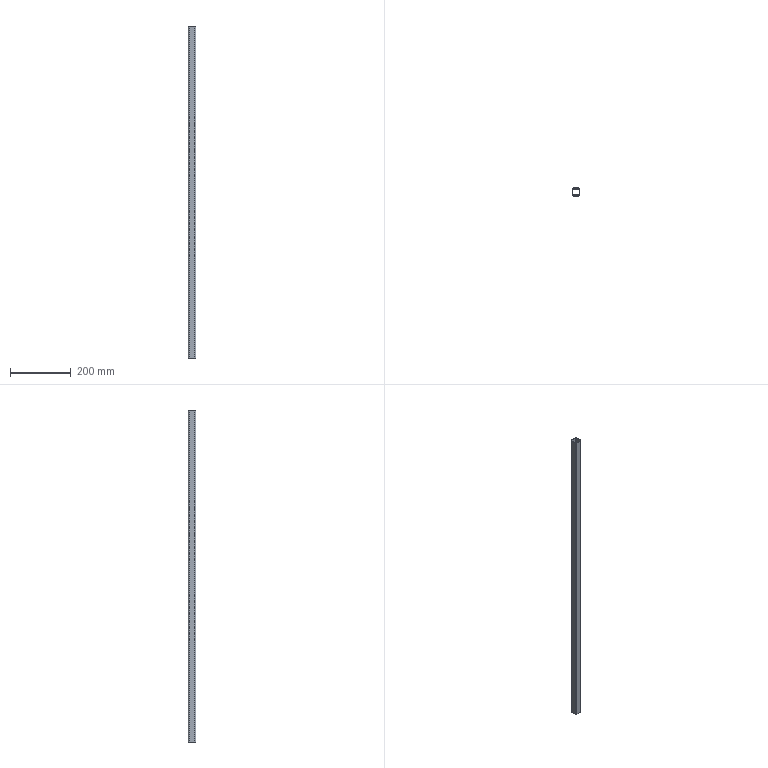Part | SolidWorks | features Extrusion 1 | 1 solid | 18 faces | box 25 x 25 x 1094 mm | volume 190027 mm3 | plane 10 | cylinder 8 | commonest cylinder face diameters 4 x4 8 x4
STEP:
#1=CARTESIAN_POINT('',(12.5,8.5,1094.));
#2=VERTEX_POINT('',#1);
#3=CARTESIAN_POINT('',(8.5,12.5,1094.));
#4=VERTEX_POINT('',#3);
#5=CARTESIAN_POINT('',(8.5,8.5,1094.));
#6=DIRECTION('',(0.,0.,1.));
#7=DIRECTION('',(1.,0.,0.));
#8=AXIS2_PLACEMENT_3D('',#5,#6,#7);
#9=CIRCLE('',#8,4.);
#10=EDGE_CURVE('',#2,#4,#9,.T.);
#11=ORIENTED_EDGE('',*,*,#10,.T.);
#12=CARTESIAN_POINT('',(-8.5,12.5,1094.));
#13=VERTEX_POINT('',#12);
#14=CARTESIAN_POINT('',(8.5,12.5,1094.));
#15=DIRECTION('',(-1.,0.,0.));
#16=VECTOR('',#15,1000.);
#17=LINE('',#14,#16);
#18=EDGE_CURVE('',#4,#13,#17,.T.);
#19=ORIENTED_EDGE('',*,*,#18,.T.);
#20=CARTESIAN_POINT('',(-12.5,8.5,1094.));
#21=VERTEX_POINT('',#20);
#22=CARTESIAN_POINT('',(-8.5,8.5,1094.));
#23=DIRECTION('',(0.,0.,1.));
#24=DIRECTION('',(1.,0.,0.));
#25=AXIS2_PLACEMENT_3D('',#22,#23,#24);
#26=CIRCLE('',#25,4.);
#27=EDGE_CURVE('',#13,#21,#26,.T.);
#28=ORIENTED_EDGE('',*,*,#27,.T.);
#29=CARTESIAN_POINT('',(-12.5,-8.5,1094.));
#30=VERTEX_POINT('',#29);
#31=CARTESIAN_POINT('',(-12.5,-8.5,1094.));
#32=DIRECTION('',(0.,-1.,0.));
#33=VECTOR('',#32,1000.);
#34=LINE('',#31,#33);
#35=EDGE_CURVE('',#21,#30,#34,.T.);
#36=ORIENTED_EDGE('',*,*,#35,.T.);
#37=CARTESIAN_POINT('',(-8.5,-12.5,1094.));
#38=VERTEX_POINT('',#37);
#39=CARTESIAN_POINT('',(-8.5,-8.5,1094.));
#40=DIRECTION('',(0.,0.,1.));
#41=DIRECTION('',(1.,0.,0.));
#42=AXIS2_PLACEMENT_3D('',#39,#40,#41);
#43=CIRCLE('',#42,4.);
#44=EDGE_CURVE('',#30,#38,#43,.T.);
#45=ORIENTED_EDGE('',*,*,#44,.T.);
#46=CARTESIAN_POINT('',(8.5,-12.5,1094.));
#47=VERTEX_POINT('',#46);
#48=CARTESIAN_POINT('',(-8.5,-12.5,1094.));
#49=DIRECTION('',(1.,0.,0.));
#50=VECTOR('',#49,1000.);
#51=LINE('',#48,#50);
#52=EDGE_CURVE('',#38,#47,#51,.T.);
#53=ORIENTED_EDGE('',*,*,#52,.T.);
#54=CARTESIAN_POINT('',(12.5,-8.5,1094.));
#55=VERTEX_POINT('',#54);
#56=CARTESIAN_POINT('',(8.5,-8.5,1094.));
#57=DIRECTION('',(0.,0.,1.));
#58=DIRECTION('',(1.,0.,0.));
#59=AXIS2_PLACEMENT_3D('',#56,#57,#58);
#60=CIRCLE('',#59,4.);
#61=EDGE_CURVE('',#47,#55,#60,.T.);
#62=ORIENTED_EDGE('',*,*,#61,.T.);
#63=CARTESIAN_POINT('',(12.5,8.5,1094.));
#64=DIRECTION('',(0.,1.,0.));
#65=VECTOR('',#64,1000.);
#66=LINE('',#63,#65);
#67=EDGE_CURVE('',#55,#2,#66,.T.);
#68=ORIENTED_EDGE('',*,*,#67,.T.);
#69=EDGE_LOOP('',(#11,#19,#28,#36,#45,#53,#62,#68));
#70=FACE_OUTER_BOUND('',#69,.T.);
#71=CARTESIAN_POINT('',(-10.5,8.5,1094.));
#72=VERTEX_POINT('',#71);
#73=CARTESIAN_POINT('',(-10.5,-8.5,1094.));
#74=VERTEX_POINT('',#73);
#75=CARTESIAN_POINT('',(-10.5,-8.5,1094.));
#76=DIRECTION('',(0.,-1.,0.));
#77=VECTOR('',#76,1000.);
#78=LINE('',#75,#77);
#79=EDGE_CURVE('',#72,#74,#78,.T.);
#80=ORIENTED_EDGE('',*,*,#79,.F.);
#81=CARTESIAN_POINT('',(-8.5,10.5,1094.));
#82=VERTEX_POINT('',#81);
#83=CARTESIAN_POINT('',(-8.5,8.5,1094.));
#84=DIRECTION('',(0.,0.,1.));
#85=DIRECTION('',(1.,0.,0.));
#86=AXIS2_PLACEMENT_3D('',#83,#84,#85);
#87=CIRCLE('',#86,2.);
#88=EDGE_CURVE('',#82,#72,#87,.T.);
#89=ORIENTED_EDGE('',*,*,#88,.F.);
#90=CARTESIAN_POINT('',(8.5,10.5,1094.));
#91=VERTEX_POINT('',#90);
#92=CARTESIAN_POINT('',(8.5,10.5,1094.));
#93=DIRECTION('',(-1.,0.,0.));
#94=VECTOR('',#93,1000.);
#95=LINE('',#92,#94);
#96=EDGE_CURVE('',#91,#82,#95,.T.);
#97=ORIENTED_EDGE('',*,*,#96,.F.);
#98=CARTESIAN_POINT('',(10.5,8.5,1094.));
#99=VERTEX_POINT('',#98);
#100=CARTESIAN_POINT('',(8.5,8.5,1094.));
#101=DIRECTION('',(0.,0.,1.));
#102=DIRECTION('',(1.,0.,0.));
#103=AXIS2_PLACEMENT_3D('',#100,#101,#102);
#104=CIRCLE('',#103,2.);
#105=EDGE_CURVE('',#99,#91,#104,.T.);
#106=ORIENTED_EDGE('',*,*,#105,.F.);
#107=CARTESIAN_POINT('',(10.5,-8.5,1094.));
#108=VERTEX_POINT('',#107);
#109=CARTESIAN_POINT('',(10.5,8.5,1094.));
#110=DIRECTION('',(0.,1.,0.));
#111=VECTOR('',#110,1000.);
#112=LINE('',#109,#111);
#113=EDGE_CURVE('',#108,#99,#112,.T.);
#114=ORIENTED_EDGE('',*,*,#113,.F.);
#115=CARTESIAN_POINT('',(8.5,-10.5,1094.));
#116=VERTEX_POINT('',#115);
#117=CARTESIAN_POINT('',(8.5,-8.5,1094.));
#118=DIRECTION('',(0.,0.,1.));
#119=DIRECTION('',(1.,0.,0.));
#120=AXIS2_PLACEMENT_3D('',#117,#118,#119);
#121=CIRCLE('',#120,2.);
#122=EDGE_CURVE('',#116,#108,#121,.T.);
#123=ORIENTED_EDGE('',*,*,#122,.F.);
#124=CARTESIAN_POINT('',(-8.5,-10.5,1094.));
#125=VERTEX_POINT('',#124);
#126=CARTESIAN_POINT('',(-8.5,-10.5,1094.));
#127=DIRECTION('',(1.,0.,0.));
#128=VECTOR('',#127,1000.);
#129=LINE('',#126,#128);
#130=EDGE_CURVE('',#125,#116,#129,.T.);
#131=ORIENTED_EDGE('',*,*,#130,.F.);
#132=CARTESIAN_POINT('',(-8.5,-8.5,1094.));
#133=DIRECTION('',(0.,0.,1.));
#134=DIRECTION('',(1.,0.,0.));
#135=AXIS2_PLACEMENT_3D('',#132,#133,#134);
#136=CIRCLE('',#135,2.);
#137=EDGE_CURVE('',#74,#125,#136,.T.);
#138=ORIENTED_EDGE('',*,*,#137,.F.);
#139=EDGE_LOOP('',(#80,#89,#97,#106,#114,#123,#131,#138));
#140=FACE_BOUND('',#139,.T.);
#141=CARTESIAN_POINT('',(8.5,8.5,1094.));
#142=DIRECTION('',(0.,0.,1.));
#143=DIRECTION('',(1.,0.,0.));
#144=AXIS2_PLACEMENT_3D('',#141,#142,#143);
#145=PLANE('',#144);
#146=ADVANCED_FACE('',(#70,#140),#145,.T.);
#147=CARTESIAN_POINT('',(12.5,8.5,0.));
#148=VERTEX_POINT('',#147);
#149=CARTESIAN_POINT('',(8.5,12.5,0.));
#150=VERTEX_POINT('',#149);
#151=CARTESIAN_POINT('',(8.5,8.5,0.));
#152=DIRECTION('',(0.,0.,1.));
#153=DIRECTION('',(1.,0.,0.));
#154=AXIS2_PLACEMENT_3D('',#151,#152,#153);
#155=CIRCLE('',#154,4.);
#156=EDGE_CURVE('',#148,#150,#155,.T.);
#157=ORIENTED_EDGE('',*,*,#156,.F.);
#158=CARTESIAN_POINT('',(12.5,-8.5,0.));
#159=VERTEX_POINT('',#158);
#160=CARTESIAN_POINT('',(12.5,8.5,0.));
#161=DIRECTION('',(0.,1.,0.));
#162=VECTOR('',#161,1000.);
#163=LINE('',#160,#162);
#164=EDGE_CURVE('',#159,#148,#163,.T.);
#165=ORIENTED_EDGE('',*,*,#164,.F.);
#166=CARTESIAN_POINT('',(8.5,-12.5,0.));
#167=VERTEX_POINT('',#166);
#168=CARTESIAN_POINT('',(8.5,-8.5,0.));
#169=DIRECTION('',(0.,0.,1.));
#170=DIRECTION('',(1.,0.,0.));
#171=AXIS2_PLACEMENT_3D('',#168,#169,#170);
#172=CIRCLE('',#171,4.);
#173=EDGE_CURVE('',#167,#159,#172,.T.);
#174=ORIENTED_EDGE('',*,*,#173,.F.);
#175=CARTESIAN_POINT('',(-8.5,-12.5,0.));
#176=VERTEX_POINT('',#175);
#177=CARTESIAN_POINT('',(-8.5,-12.5,0.));
#178=DIRECTION('',(1.,0.,0.));
#179=VECTOR('',#178,1000.);
#180=LINE('',#177,#179);
#181=EDGE_CURVE('',#176,#167,#180,.T.);
#182=ORIENTED_EDGE('',*,*,#181,.F.);
#183=CARTESIAN_POINT('',(-12.5,-8.5,0.));
#184=VERTEX_POINT('',#183);
#185=CARTESIAN_POINT('',(-8.5,-8.5,0.));
#186=DIRECTION('',(0.,0.,1.));
#187=DIRECTION('',(1.,0.,0.));
#188=AXIS2_PLACEMENT_3D('',#185,#186,#187);
#189=CIRCLE('',#188,4.);
#190=EDGE_CURVE('',#184,#176,#189,.T.);
#191=ORIENTED_EDGE('',*,*,#190,.F.);
#192=CARTESIAN_POINT('',(-12.5,8.5,0.));
#193=VERTEX_POINT('',#192);
#194=CARTESIAN_POINT('',(-12.5,-8.5,0.));
#195=DIRECTION('',(0.,-1.,0.));
#196=VECTOR('',#195,1000.);
#197=LINE('',#194,#196);
#198=EDGE_CURVE('',#193,#184,#197,.T.);
#199=ORIENTED_EDGE('',*,*,#198,.F.);
#200=CARTESIAN_POINT('',(-8.5,12.5,0.));
#201=VERTEX_POINT('',#200);
#202=CARTESIAN_POINT('',(-8.5,8.5,0.));
#203=DIRECTION('',(0.,0.,1.));
#204=DIRECTION('',(1.,0.,0.));
#205=AXIS2_PLACEMENT_3D('',#202,#203,#204);
#206=CIRCLE('',#205,4.);
#207=EDGE_CURVE('',#201,#193,#206,.T.);
#208=ORIENTED_EDGE('',*,*,#207,.F.);
#209=CARTESIAN_POINT('',(8.5,12.5,0.));
#210=DIRECTION('',(-1.,0.,0.));
#211=VECTOR('',#210,1000.);
#212=LINE('',#209,#211);
#213=EDGE_CURVE('',#150,#201,#212,.T.);
#214=ORIENTED_EDGE('',*,*,#213,.F.);
#215=EDGE_LOOP('',(#157,#165,#174,#182,#191,#199,#208,#214));
#216=FACE_OUTER_BOUND('',#215,.T.);
#217=CARTESIAN_POINT('',(-8.5,10.5,0.));
#218=VERTEX_POINT('',#217);
#219=CARTESIAN_POINT('',(-10.5,8.5,0.));
#220=VERTEX_POINT('',#219);
#221=CARTESIAN_POINT('',(-8.5,8.5,0.));
#222=DIRECTION('',(0.,0.,1.));
#223=DIRECTION('',(1.,0.,0.));
#224=AXIS2_PLACEMENT_3D('',#221,#222,#223);
#225=CIRCLE('',#224,2.);
#226=EDGE_CURVE('',#218,#220,#225,.T.);
#227=ORIENTED_EDGE('',*,*,#226,.T.);
#228=CARTESIAN_POINT('',(-10.5,-8.5,0.));
#229=VERTEX_POINT('',#228);
#230=CARTESIAN_POINT('',(-10.5,-8.5,0.));
#231=DIRECTION('',(0.,-1.,0.));
#232=VECTOR('',#231,1000.);
#233=LINE('',#230,#232);
#234=EDGE_CURVE('',#220,#229,#233,.T.);
#235=ORIENTED_EDGE('',*,*,#234,.T.);
#236=CARTESIAN_POINT('',(-8.5,-10.5,0.));
#237=VERTEX_POINT('',#236);
#238=CARTESIAN_POINT('',(-8.5,-8.5,0.));
#239=DIRECTION('',(0.,0.,1.));
#240=DIRECTION('',(1.,0.,0.));
#241=AXIS2_PLACEMENT_3D('',#238,#239,#240);
#242=CIRCLE('',#241,2.);
#243=EDGE_CURVE('',#229,#237,#242,.T.);
#244=ORIENTED_EDGE('',*,*,#243,.T.);
#245=CARTESIAN_POINT('',(8.5,-10.5,0.));
#246=VERTEX_POINT('',#245);
#247=CARTESIAN_POINT('',(-8.5,-10.5,0.));
#248=DIRECTION('',(1.,0.,0.));
#249=VECTOR('',#248,1000.);
#250=LINE('',#247,#249);
#251=EDGE_CURVE('',#237,#246,#250,.T.);
#252=ORIENTED_EDGE('',*,*,#251,.T.);
#253=CARTESIAN_POINT('',(10.5,-8.5,0.));
#254=VERTEX_POINT('',#253);
#255=CARTESIAN_POINT('',(8.5,-8.5,0.));
#256=DIRECTION('',(0.,0.,1.));
#257=DIRECTION('',(1.,0.,0.));
#258=AXIS2_PLACEMENT_3D('',#255,#256,#257);
#259=CIRCLE('',#258,2.);
#260=EDGE_CURVE('',#246,#254,#259,.T.);
#261=ORIENTED_EDGE('',*,*,#260,.T.);
#262=CARTESIAN_POINT('',(10.5,8.5,0.));
#263=VERTEX_POINT('',#262);
#264=CARTESIAN_POINT('',(10.5,8.5,0.));
#265=DIRECTION('',(0.,1.,0.));
#266=VECTOR('',#265,1000.);
#267=LINE('',#264,#266);
#268=EDGE_CURVE('',#254,#263,#267,.T.);
#269=ORIENTED_EDGE('',*,*,#268,.T.);
#270=CARTESIAN_POINT('',(8.5,10.5,0.));
#271=VERTEX_POINT('',#270);
#272=CARTESIAN_POINT('',(8.5,8.5,0.));
#273=DIRECTION('',(0.,0.,1.));
#274=DIRECTION('',(1.,0.,0.));
#275=AXIS2_PLACEMENT_3D('',#272,#273,#274);
#276=CIRCLE('',#275,2.);
#277=EDGE_CURVE('',#263,#271,#276,.T.);
#278=ORIENTED_EDGE('',*,*,#277,.T.);
#279=CARTESIAN_POINT('',(8.5,10.5,0.));
#280=DIRECTION('',(-1.,0.,0.));
#281=VECTOR('',#280,1000.);
#282=LINE('',#279,#281);
#283=EDGE_CURVE('',#271,#218,#282,.T.);
#284=ORIENTED_EDGE('',*,*,#283,.T.);
#285=EDGE_LOOP('',(#227,#235,#244,#252,#261,#269,#278,#284));
#286=FACE_BOUND('',#285,.T.);
#287=CARTESIAN_POINT('',(8.5,8.5,0.));
#288=DIRECTION('',(0.,0.,1.));
#289=DIRECTION('',(1.,0.,0.));
#290=AXIS2_PLACEMENT_3D('',#287,#288,#289);
#291=PLANE('',#290);
#292=ADVANCED_FACE('',(#216,#286),#291,.F.);
#293=ORIENTED_EDGE('',*,*,#156,.T.);
#294=CARTESIAN_POINT('',(8.5,12.5,1094.));
#295=DIRECTION('',(0.,0.,-1.));
#296=VECTOR('',#295,1000.);
#297=LINE('',#294,#296);
#298=EDGE_CURVE('',#4,#150,#297,.T.);
#299=ORIENTED_EDGE('',*,*,#298,.F.);
#300=ORIENTED_EDGE('',*,*,#10,.F.);
#301=CARTESIAN_POINT('',(12.5,8.5,1094.));
#302=DIRECTION('',(0.,0.,-1.));
#303=VECTOR('',#302,1000.);
#304=LINE('',#301,#303);
#305=EDGE_CURVE('',#2,#148,#304,.T.);
#306=ORIENTED_EDGE('',*,*,#305,.T.);
#307=EDGE_LOOP('',(#293,#299,#300,#306));
#308=FACE_OUTER_BOUND('',#307,.T.);
#309=CARTESIAN_POINT('',(8.5,8.5,1094.));
#310=DIRECTION('',(0.,0.,-1.));
#311=DIRECTION('',(-1.,0.,0.));
#312=AXIS2_PLACEMENT_3D('',#309,#310,#311);
#313=CYLINDRICAL_SURFACE('',#312,4.);
#314=ADVANCED_FACE('',(#308),#313,.T.);
#315=ORIENTED_EDGE('',*,*,#213,.T.);
#316=CARTESIAN_POINT('',(-8.5,12.5,1094.));
#317=DIRECTION('',(0.,0.,-1.));
#318=VECTOR('',#317,1000.);
#319=LINE('',#316,#318);
#320=EDGE_CURVE('',#13,#201,#319,.T.);
#321=ORIENTED_EDGE('',*,*,#320,.F.);
#322=ORIENTED_EDGE('',*,*,#18,.F.);
#323=ORIENTED_EDGE('',*,*,#298,.T.);
#324=EDGE_LOOP('',(#315,#321,#322,#323));
#325=FACE_OUTER_BOUND('',#324,.T.);
#326=CARTESIAN_POINT('',(8.5,12.5,1094.));
#327=DIRECTION('',(0.,-1.,0.));
#328=DIRECTION('',(0.,0.,-1.));
#329=AXIS2_PLACEMENT_3D('',#326,#327,#328);
#330=PLANE('',#329);
#331=ADVANCED_FACE('',(#325),#330,.F.);
#332=ORIENTED_EDGE('',*,*,#207,.T.);
#333=CARTESIAN_POINT('',(-12.5,8.5,1094.));
#334=DIRECTION('',(0.,0.,-1.));
#335=VECTOR('',#334,1000.);
#336=LINE('',#333,#335);
#337=EDGE_CURVE('',#21,#193,#336,.T.);
#338=ORIENTED_EDGE('',*,*,#337,.F.);
#339=ORIENTED_EDGE('',*,*,#27,.F.);
#340=ORIENTED_EDGE('',*,*,#320,.T.);
#341=EDGE_LOOP('',(#332,#338,#339,#340));
#342=FACE_OUTER_BOUND('',#341,.T.);
#343=CARTESIAN_POINT('',(-8.5,8.5,1094.));
#344=DIRECTION('',(0.,0.,-1.));
#345=DIRECTION('',(-1.,0.,0.));
#346=AXIS2_PLACEMENT_3D('',#343,#344,#345);
#347=CYLINDRICAL_SURFACE('',#346,4.);
#348=ADVANCED_FACE('',(#342),#347,.T.);
#349=ORIENTED_EDGE('',*,*,#198,.T.);
#350=CARTESIAN_POINT('',(-12.5,-8.5,1094.));
#351=DIRECTION('',(0.,0.,-1.));
#352=VECTOR('',#351,1000.);
#353=LINE('',#350,#352);
#354=EDGE_CURVE('',#30,#184,#353,.T.);
#355=ORIENTED_EDGE('',*,*,#354,.F.);
#356=ORIENTED_EDGE('',*,*,#35,.F.);
#357=ORIENTED_EDGE('',*,*,#337,.T.);
#358=EDGE_LOOP('',(#349,#355,#356,#357));
#359=FACE_OUTER_BOUND('',#358,.T.);
#360=CARTESIAN_POINT('',(-12.5,-8.5,1094.));
#361=DIRECTION('',(1.,0.,0.));
#362=DIRECTION('',(0.,0.,-1.));
#363=AXIS2_PLACEMENT_3D('',#360,#361,#362);
#364=PLANE('',#363);
#365=ADVANCED_FACE('',(#359),#364,.F.);
#366=ORIENTED_EDGE('',*,*,#190,.T.);
#367=CARTESIAN_POINT('',(-8.5,-12.5,1094.));
#368=DIRECTION('',(0.,0.,-1.));
#369=VECTOR('',#368,1000.);
#370=LINE('',#367,#369);
#371=EDGE_CURVE('',#38,#176,#370,.T.);
#372=ORIENTED_EDGE('',*,*,#371,.F.);
#373=ORIENTED_EDGE('',*,*,#44,.F.);
#374=ORIENTED_EDGE('',*,*,#354,.T.);
#375=EDGE_LOOP('',(#366,#372,#373,#374));
#376=FACE_OUTER_BOUND('',#375,.T.);
#377=CARTESIAN_POINT('',(-8.5,-8.5,1094.));
#378=DIRECTION('',(0.,0.,-1.));
#379=DIRECTION('',(-1.,0.,0.));
#380=AXIS2_PLACEMENT_3D('',#377,#378,#379);
#381=CYLINDRICAL_SURFACE('',#380,4.);
#382=ADVANCED_FACE('',(#376),#381,.T.);
#383=ORIENTED_EDGE('',*,*,#181,.T.);
#384=CARTESIAN_POINT('',(8.5,-12.5,1094.));
#385=DIRECTION('',(0.,0.,-1.));
#386=VECTOR('',#385,1000.);
#387=LINE('',#384,#386);
#388=EDGE_CURVE('',#47,#167,#387,.T.);
#389=ORIENTED_EDGE('',*,*,#388,.F.);
#390=ORIENTED_EDGE('',*,*,#52,.F.);
#391=ORIENTED_EDGE('',*,*,#371,.T.);
#392=EDGE_LOOP('',(#383,#389,#390,#391));
#393=FACE_OUTER_BOUND('',#392,.T.);
#394=CARTESIAN_POINT('',(-8.5,-12.5,1094.));
#395=DIRECTION('',(0.,1.,0.));
#396=DIRECTION('',(0.,0.,1.));
#397=AXIS2_PLACEMENT_3D('',#394,#395,#396);
#398=PLANE('',#397);
#399=ADVANCED_FACE('',(#393),#398,.F.);
#400=ORIENTED_EDGE('',*,*,#173,.T.);
#401=CARTESIAN_POINT('',(12.5,-8.5,1094.));
#402=DIRECTION('',(0.,0.,-1.));
#403=VECTOR('',#402,1000.);
#404=LINE('',#401,#403);
#405=EDGE_CURVE('',#55,#159,#404,.T.);
#406=ORIENTED_EDGE('',*,*,#405,.F.);
#407=ORIENTED_EDGE('',*,*,#61,.F.);
#408=ORIENTED_EDGE('',*,*,#388,.T.);
#409=EDGE_LOOP('',(#400,#406,#407,#408));
#410=FACE_OUTER_BOUND('',#409,.T.);
#411=CARTESIAN_POINT('',(8.5,-8.5,1094.));
#412=DIRECTION('',(0.,0.,-1.));
#413=DIRECTION('',(-1.,0.,0.));
#414=AXIS2_PLACEMENT_3D('',#411,#412,#413);
#415=CYLINDRICAL_SURFACE('',#414,4.);
#416=ADVANCED_FACE('',(#410),#415,.T.);
#417=ORIENTED_EDGE('',*,*,#164,.T.);
#418=ORIENTED_EDGE('',*,*,#305,.F.);
#419=ORIENTED_EDGE('',*,*,#67,.F.);
#420=ORIENTED_EDGE('',*,*,#405,.T.);
#421=EDGE_LOOP('',(#417,#418,#419,#420));
#422=FACE_OUTER_BOUND('',#421,.T.);
#423=CARTESIAN_POINT('',(12.5,8.5,1094.));
#424=DIRECTION('',(-1.,0.,0.));
#425=DIRECTION('',(0.,0.,1.));
#426=AXIS2_PLACEMENT_3D('',#423,#424,#425);
#427=PLANE('',#426);
#428=ADVANCED_FACE('',(#422),#427,.F.);
#429=ORIENTED_EDGE('',*,*,#226,.F.);
#430=CARTESIAN_POINT('',(-8.5,10.5,1094.));
#431=DIRECTION('',(0.,0.,-1.));
#432=VECTOR('',#431,1000.);
#433=LINE('',#430,#432);
#434=EDGE_CURVE('',#82,#218,#433,.T.);
#435=ORIENTED_EDGE('',*,*,#434,.F.);
#436=ORIENTED_EDGE('',*,*,#88,.T.);
#437=CARTESIAN_POINT('',(-10.5,8.5,1094.));
#438=DIRECTION('',(0.,0.,-1.));
#439=VECTOR('',#438,1000.);
#440=LINE('',#437,#439);
#441=EDGE_CURVE('',#72,#220,#440,.T.);
#442=ORIENTED_EDGE('',*,*,#441,.T.);
#443=EDGE_LOOP('',(#429,#435,#436,#442));
#444=FACE_OUTER_BOUND('',#443,.T.);
#445=CARTESIAN_POINT('',(-8.5,8.5,1094.));
#446=DIRECTION('',(0.,0.,-1.));
#447=DIRECTION('',(-1.,0.,0.));
#448=AXIS2_PLACEMENT_3D('',#445,#446,#447);
#449=CYLINDRICAL_SURFACE('',#448,2.);
#450=ADVANCED_FACE('',(#444),#449,.F.);
#451=ORIENTED_EDGE('',*,*,#234,.F.);
#452=ORIENTED_EDGE('',*,*,#441,.F.);
#453=ORIENTED_EDGE('',*,*,#79,.T.);
#454=CARTESIAN_POINT('',(-10.5,-8.5,1094.));
#455=DIRECTION('',(0.,0.,-1.));
#456=VECTOR('',#455,1000.);
#457=LINE('',#454,#456);
#458=EDGE_CURVE('',#74,#229,#457,.T.);
#459=ORIENTED_EDGE('',*,*,#458,.T.);
#460=EDGE_LOOP('',(#451,#452,#453,#459));
#461=FACE_OUTER_BOUND('',#460,.T.);
#462=CARTESIAN_POINT('',(-10.5,-8.5,1094.));
#463=DIRECTION('',(1.,0.,0.));
#464=DIRECTION('',(0.,0.,-1.));
#465=AXIS2_PLACEMENT_3D('',#462,#463,#464);
#466=PLANE('',#465);
#467=ADVANCED_FACE('',(#461),#466,.T.);
#468=ORIENTED_EDGE('',*,*,#243,.F.);
#469=ORIENTED_EDGE('',*,*,#458,.F.);
#470=ORIENTED_EDGE('',*,*,#137,.T.);
#471=CARTESIAN_POINT('',(-8.5,-10.5,1094.));
#472=DIRECTION('',(0.,0.,-1.));
#473=VECTOR('',#472,1000.);
#474=LINE('',#471,#473);
#475=EDGE_CURVE('',#125,#237,#474,.T.);
#476=ORIENTED_EDGE('',*,*,#475,.T.);
#477=EDGE_LOOP('',(#468,#469,#470,#476));
#478=FACE_OUTER_BOUND('',#477,.T.);
#479=CARTESIAN_POINT('',(-8.5,-8.5,1094.));
#480=DIRECTION('',(0.,0.,-1.));
#481=DIRECTION('',(-1.,0.,0.));
#482=AXIS2_PLACEMENT_3D('',#479,#480,#481);
#483=CYLINDRICAL_SURFACE('',#482,2.);
#484=ADVANCED_FACE('',(#478),#483,.F.);
#485=ORIENTED_EDGE('',*,*,#251,.F.);
#486=ORIENTED_EDGE('',*,*,#475,.F.);
#487=ORIENTED_EDGE('',*,*,#130,.T.);
#488=CARTESIAN_POINT('',(8.5,-10.5,1094.));
#489=DIRECTION('',(0.,0.,-1.));
#490=VECTOR('',#489,1000.);
#491=LINE('',#488,#490);
#492=EDGE_CURVE('',#116,#246,#491,.T.);
#493=ORIENTED_EDGE('',*,*,#492,.T.);
#494=EDGE_LOOP('',(#485,#486,#487,#493));
#495=FACE_OUTER_BOUND('',#494,.T.);
#496=CARTESIAN_POINT('',(-8.5,-10.5,1094.));
#497=DIRECTION('',(0.,1.,0.));
#498=DIRECTION('',(0.,0.,1.));
#499=AXIS2_PLACEMENT_3D('',#496,#497,#498);
#500=PLANE('',#499);
#501=ADVANCED_FACE('',(#495),#500,.T.);
#502=ORIENTED_EDGE('',*,*,#260,.F.);
#503=ORIENTED_EDGE('',*,*,#492,.F.);
#504=ORIENTED_EDGE('',*,*,#122,.T.);
#505=CARTESIAN_POINT('',(10.5,-8.5,1094.));
#506=DIRECTION('',(0.,0.,-1.));
#507=VECTOR('',#506,1000.);
#508=LINE('',#505,#507);
#509=EDGE_CURVE('',#108,#254,#508,.T.);
#510=ORIENTED_EDGE('',*,*,#509,.T.);
#511=EDGE_LOOP('',(#502,#503,#504,#510));
#512=FACE_OUTER_BOUND('',#511,.T.);
#513=CARTESIAN_POINT('',(8.5,-8.5,1094.));
#514=DIRECTION('',(0.,0.,-1.));
#515=DIRECTION('',(-1.,0.,0.));
#516=AXIS2_PLACEMENT_3D('',#513,#514,#515);
#517=CYLINDRICAL_SURFACE('',#516,2.);
#518=ADVANCED_FACE('',(#512),#517,.F.);
#519=ORIENTED_EDGE('',*,*,#268,.F.);
#520=ORIENTED_EDGE('',*,*,#509,.F.);
#521=ORIENTED_EDGE('',*,*,#113,.T.);
#522=CARTESIAN_POINT('',(10.5,8.5,1094.));
#523=DIRECTION('',(0.,0.,-1.));
#524=VECTOR('',#523,1000.);
#525=LINE('',#522,#524);
#526=EDGE_CURVE('',#99,#263,#525,.T.);
#527=ORIENTED_EDGE('',*,*,#526,.T.);
#528=EDGE_LOOP('',(#519,#520,#521,#527));
#529=FACE_OUTER_BOUND('',#528,.T.);
#530=CARTESIAN_POINT('',(10.5,8.5,1094.));
#531=DIRECTION('',(-1.,0.,0.));
#532=DIRECTION('',(0.,0.,1.));
#533=AXIS2_PLACEMENT_3D('',#530,#531,#532);
#534=PLANE('',#533);
#535=ADVANCED_FACE('',(#529),#534,.T.);
#536=ORIENTED_EDGE('',*,*,#277,.F.);
#537=ORIENTED_EDGE('',*,*,#526,.F.);
#538=ORIENTED_EDGE('',*,*,#105,.T.);
#539=CARTESIAN_POINT('',(8.5,10.5,1094.));
#540=DIRECTION('',(0.,0.,-1.));
#541=VECTOR('',#540,1000.);
#542=LINE('',#539,#541);
#543=EDGE_CURVE('',#91,#271,#542,.T.);
#544=ORIENTED_EDGE('',*,*,#543,.T.);
#545=EDGE_LOOP('',(#536,#537,#538,#544));
#546=FACE_OUTER_BOUND('',#545,.T.);
#547=CARTESIAN_POINT('',(8.5,8.5,1094.));
#548=DIRECTION('',(0.,0.,-1.));
#549=DIRECTION('',(-1.,0.,0.));
#550=AXIS2_PLACEMENT_3D('',#547,#548,#549);
#551=CYLINDRICAL_SURFACE('',#550,2.);
#552=ADVANCED_FACE('',(#546),#551,.F.);
#553=ORIENTED_EDGE('',*,*,#283,.F.);
#554=ORIENTED_EDGE('',*,*,#543,.F.);
#555=ORIENTED_EDGE('',*,*,#96,.T.);
#556=ORIENTED_EDGE('',*,*,#434,.T.);
#557=EDGE_LOOP('',(#553,#554,#555,#556));
#558=FACE_OUTER_BOUND('',#557,.T.);
#559=CARTESIAN_POINT('',(8.5,10.5,1094.));
#560=DIRECTION('',(0.,-1.,0.));
#561=DIRECTION('',(0.,0.,-1.));
#562=AXIS2_PLACEMENT_3D('',#559,#560,#561);
#563=PLANE('',#562);
#564=ADVANCED_FACE('',(#558),#563,.T.);
#565=CLOSED_SHELL('',(#146,#292,#314,#331,#348,#365,#382,#399,#416,#428,#450,#467,#484,#501,#518,#535,#552,#564));
#566=MANIFOLD_SOLID_BREP('',#565);
#567=CARTESIAN_POINT('',(0.,0.,0.));
#568=DIRECTION('',(0.,0.,1.));
#569=DIRECTION('',(1.,0.,0.));
#570=AXIS2_PLACEMENT_3D('',#567,#568,#569);
#571=(LENGTH_UNIT()NAMED_UNIT(*)SI_UNIT(.MILLI.,.METRE.));
#572=UNCERTAINTY_MEASURE_WITH_UNIT(LENGTH_MEASURE(0.00001),#571,'','');
#573=(NAMED_UNIT(*)PLANE_ANGLE_UNIT()SI_UNIT($,.RADIAN.));
#574=(NAMED_UNIT(*)SI_UNIT($,.STERADIAN.)SOLID_ANGLE_UNIT());
#575=(GEOMETRIC_REPRESENTATION_CONTEXT(3)GLOBAL_UNCERTAINTY_ASSIGNED_CONTEXT((#572))GLOBAL_UNIT_ASSIGNED_CONTEXT((#571,#573,#574))REPRESENTATION_CONTEXT('',''));
#576=ADVANCED_BREP_SHAPE_REPRESENTATION('',(#566,#570),#575);